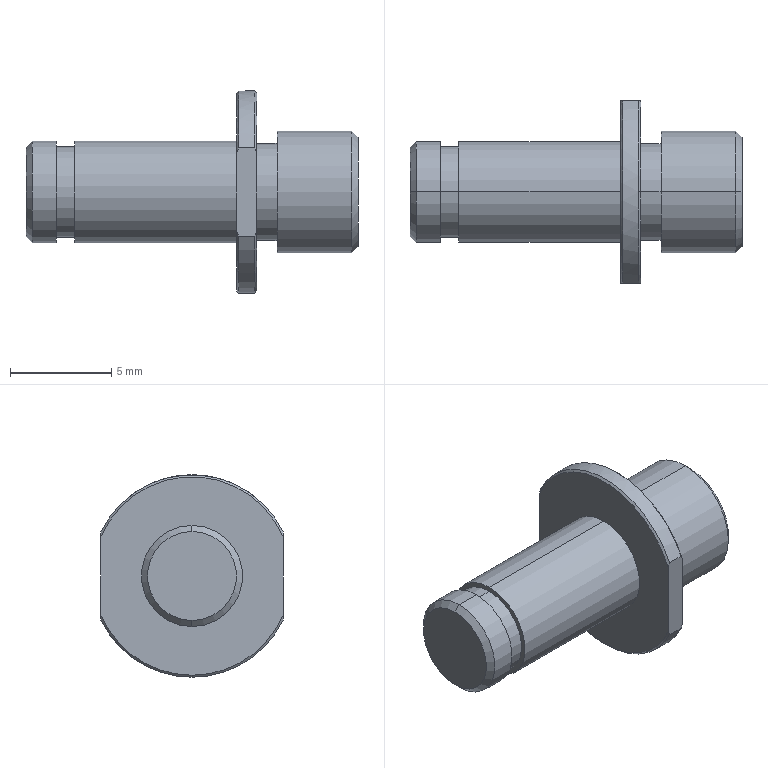Part | STEP file | Transition Guide Wheel Axle | 1 solid | 32 faces | box 16.4 x 9 x 10 mm | volume 405.919 mm3 | cylinder 13 | cone 10 | plane 9 | commonest cylinder face diameters 5 x4 10 x3 4.5 x2 4.8 x2 6 x2